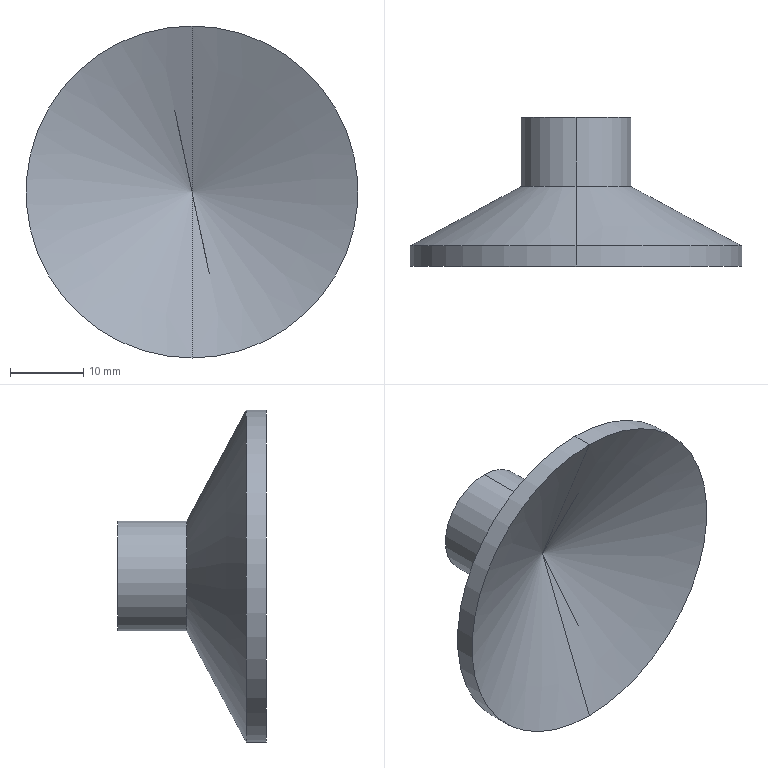Part | SolidWorks | features BaseBody 1 | 1 solid | 14 faces | box 45.38 x 20.336 x 45.38 mm | volume 6966 mm3 | plane 6 | cylinder 4 | cone 4 | commonest cylinder face diameters 15.016 x2 45.38 x2